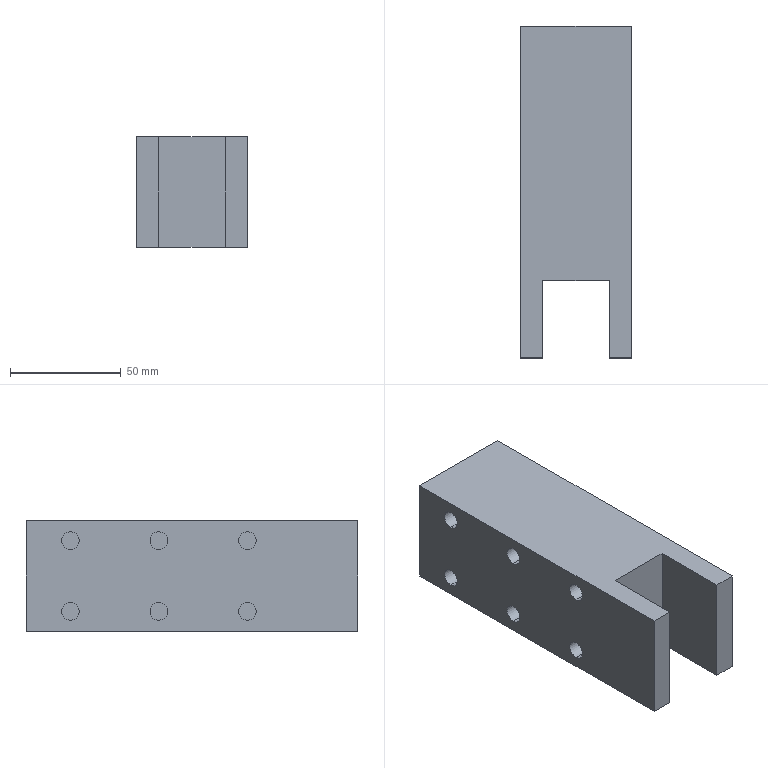Part | SolidWorks | features ICE 3, Extrusion 1, MirrorPattern 1 | 1 solid | 49 faces | box 50 x 150 x 50 mm | volume 308426 mm3 | cylinder 26 | plane 23 | commonest cylinder face diameters 8 x24 32 x2
STEP:
#1=CARTESIAN_POINT('',(-15.,130.,-20.));
#2=VERTEX_POINT('',#1);
#3=CARTESIAN_POINT('',(-15.,130.,-12.));
#4=VERTEX_POINT('',#3);
#5=CARTESIAN_POINT('',(-15.,130.,-16.));
#6=DIRECTION('',(-1.,0.,0.));
#7=DIRECTION('',(0.,0.,-1.));
#8=AXIS2_PLACEMENT_3D('',#5,#6,#7);
#9=CIRCLE('',#8,4.);
#10=EDGE_CURVE('',#2,#4,#9,.T.);
#11=ORIENTED_EDGE('',*,*,#10,.F.);
#12=CARTESIAN_POINT('',(-25.,130.,-20.));
#13=VERTEX_POINT('',#12);
#14=CARTESIAN_POINT('',(-15.,130.,-20.));
#15=DIRECTION('',(-1.,0.,0.));
#16=VECTOR('',#15,1000.);
#17=LINE('',#14,#16);
#18=EDGE_CURVE('',#2,#13,#17,.T.);
#19=ORIENTED_EDGE('',*,*,#18,.T.);
#20=CARTESIAN_POINT('',(-25.,130.,-12.));
#21=VERTEX_POINT('',#20);
#22=CARTESIAN_POINT('',(-25.,130.,-16.));
#23=DIRECTION('',(-1.,0.,0.));
#24=DIRECTION('',(0.,0.,-1.));
#25=AXIS2_PLACEMENT_3D('',#22,#23,#24);
#26=CIRCLE('',#25,4.);
#27=EDGE_CURVE('',#13,#21,#26,.T.);
#28=ORIENTED_EDGE('',*,*,#27,.T.);
#29=CARTESIAN_POINT('',(-15.,130.,-12.));
#30=DIRECTION('',(-1.,0.,0.));
#31=VECTOR('',#30,1000.);
#32=LINE('',#29,#31);
#33=EDGE_CURVE('',#4,#21,#32,.T.);
#34=ORIENTED_EDGE('',*,*,#33,.F.);
#35=EDGE_LOOP('',(#11,#19,#28,#34));
#36=FACE_OUTER_BOUND('',#35,.T.);
#37=CARTESIAN_POINT('',(-15.,130.,-16.));
#38=DIRECTION('',(-1.,0.,0.));
#39=DIRECTION('',(0.,0.,1.));
#40=AXIS2_PLACEMENT_3D('',#37,#38,#39);
#41=CYLINDRICAL_SURFACE('',#40,4.);
#42=ADVANCED_FACE('',(#36),#41,.F.);
#43=CARTESIAN_POINT('',(-15.,90.,20.));
#44=VERTEX_POINT('',#43);
#45=CARTESIAN_POINT('',(-15.,90.,12.));
#46=VERTEX_POINT('',#45);
#47=CARTESIAN_POINT('',(-15.,90.,16.));
#48=DIRECTION('',(1.,0.,0.));
#49=DIRECTION('',(0.,0.,-1.));
#50=AXIS2_PLACEMENT_3D('',#47,#48,#49);
#51=CIRCLE('',#50,4.);
#52=EDGE_CURVE('',#44,#46,#51,.T.);
#53=ORIENTED_EDGE('',*,*,#52,.T.);
#54=CARTESIAN_POINT('',(-25.,90.,12.));
#55=VERTEX_POINT('',#54);
#56=CARTESIAN_POINT('',(-15.,90.,12.));
#57=DIRECTION('',(-1.,0.,0.));
#58=VECTOR('',#57,1000.);
#59=LINE('',#56,#58);
#60=EDGE_CURVE('',#46,#55,#59,.T.);
#61=ORIENTED_EDGE('',*,*,#60,.T.);
#62=CARTESIAN_POINT('',(-25.,90.,20.));
#63=VERTEX_POINT('',#62);
#64=CARTESIAN_POINT('',(-25.,90.,16.));
#65=DIRECTION('',(1.,0.,0.));
#66=DIRECTION('',(0.,0.,-1.));
#67=AXIS2_PLACEMENT_3D('',#64,#65,#66);
#68=CIRCLE('',#67,4.);
#69=EDGE_CURVE('',#63,#55,#68,.T.);
#70=ORIENTED_EDGE('',*,*,#69,.F.);
#71=CARTESIAN_POINT('',(-15.,90.,20.));
#72=DIRECTION('',(-1.,0.,0.));
#73=VECTOR('',#72,1000.);
#74=LINE('',#71,#73);
#75=EDGE_CURVE('',#44,#63,#74,.T.);
#76=ORIENTED_EDGE('',*,*,#75,.F.);
#77=EDGE_LOOP('',(#53,#61,#70,#76));
#78=FACE_OUTER_BOUND('',#77,.T.);
#79=CARTESIAN_POINT('',(-15.,90.,16.));
#80=DIRECTION('',(-1.,0.,0.));
#81=DIRECTION('',(0.,0.,1.));
#82=AXIS2_PLACEMENT_3D('',#79,#80,#81);
#83=CYLINDRICAL_SURFACE('',#82,4.);
#84=ADVANCED_FACE('',(#78),#83,.F.);
#85=CARTESIAN_POINT('',(-15.,50.,20.));
#86=VERTEX_POINT('',#85);
#87=CARTESIAN_POINT('',(-15.,50.,12.));
#88=VERTEX_POINT('',#87);
#89=CARTESIAN_POINT('',(-15.,50.,16.));
#90=DIRECTION('',(1.,0.,0.));
#91=DIRECTION('',(0.,0.,-1.));
#92=AXIS2_PLACEMENT_3D('',#89,#90,#91);
#93=CIRCLE('',#92,4.);
#94=EDGE_CURVE('',#86,#88,#93,.T.);
#95=ORIENTED_EDGE('',*,*,#94,.T.);
#96=CARTESIAN_POINT('',(-25.,50.,12.));
#97=VERTEX_POINT('',#96);
#98=CARTESIAN_POINT('',(-15.,50.,12.));
#99=DIRECTION('',(-1.,0.,0.));
#100=VECTOR('',#99,1000.);
#101=LINE('',#98,#100);
#102=EDGE_CURVE('',#88,#97,#101,.T.);
#103=ORIENTED_EDGE('',*,*,#102,.T.);
#104=CARTESIAN_POINT('',(-25.,50.,20.));
#105=VERTEX_POINT('',#104);
#106=CARTESIAN_POINT('',(-25.,50.,16.));
#107=DIRECTION('',(1.,0.,0.));
#108=DIRECTION('',(0.,0.,-1.));
#109=AXIS2_PLACEMENT_3D('',#106,#107,#108);
#110=CIRCLE('',#109,4.);
#111=EDGE_CURVE('',#105,#97,#110,.T.);
#112=ORIENTED_EDGE('',*,*,#111,.F.);
#113=CARTESIAN_POINT('',(-15.,50.,20.));
#114=DIRECTION('',(-1.,0.,0.));
#115=VECTOR('',#114,1000.);
#116=LINE('',#113,#115);
#117=EDGE_CURVE('',#86,#105,#116,.T.);
#118=ORIENTED_EDGE('',*,*,#117,.F.);
#119=EDGE_LOOP('',(#95,#103,#112,#118));
#120=FACE_OUTER_BOUND('',#119,.T.);
#121=CARTESIAN_POINT('',(-15.,50.,16.));
#122=DIRECTION('',(-1.,0.,0.));
#123=DIRECTION('',(0.,0.,1.));
#124=AXIS2_PLACEMENT_3D('',#121,#122,#123);
#125=CYLINDRICAL_SURFACE('',#124,4.);
#126=ADVANCED_FACE('',(#120),#125,.F.);
#127=CARTESIAN_POINT('',(-15.,50.,-20.));
#128=VERTEX_POINT('',#127);
#129=CARTESIAN_POINT('',(-15.,50.,-12.));
#130=VERTEX_POINT('',#129);
#131=CARTESIAN_POINT('',(-15.,50.,-16.));
#132=DIRECTION('',(-1.,0.,0.));
#133=DIRECTION('',(0.,0.,-1.));
#134=AXIS2_PLACEMENT_3D('',#131,#132,#133);
#135=CIRCLE('',#134,4.);
#136=EDGE_CURVE('',#128,#130,#135,.T.);
#137=ORIENTED_EDGE('',*,*,#136,.F.);
#138=CARTESIAN_POINT('',(-25.,50.,-20.));
#139=VERTEX_POINT('',#138);
#140=CARTESIAN_POINT('',(-15.,50.,-20.));
#141=DIRECTION('',(-1.,0.,0.));
#142=VECTOR('',#141,1000.);
#143=LINE('',#140,#142);
#144=EDGE_CURVE('',#128,#139,#143,.T.);
#145=ORIENTED_EDGE('',*,*,#144,.T.);
#146=CARTESIAN_POINT('',(-25.,50.,-12.));
#147=VERTEX_POINT('',#146);
#148=CARTESIAN_POINT('',(-25.,50.,-16.));
#149=DIRECTION('',(-1.,0.,0.));
#150=DIRECTION('',(0.,0.,-1.));
#151=AXIS2_PLACEMENT_3D('',#148,#149,#150);
#152=CIRCLE('',#151,4.);
#153=EDGE_CURVE('',#139,#147,#152,.T.);
#154=ORIENTED_EDGE('',*,*,#153,.T.);
#155=CARTESIAN_POINT('',(-15.,50.,-12.));
#156=DIRECTION('',(-1.,0.,0.));
#157=VECTOR('',#156,1000.);
#158=LINE('',#155,#157);
#159=EDGE_CURVE('',#130,#147,#158,.T.);
#160=ORIENTED_EDGE('',*,*,#159,.F.);
#161=EDGE_LOOP('',(#137,#145,#154,#160));
#162=FACE_OUTER_BOUND('',#161,.T.);
#163=CARTESIAN_POINT('',(-15.,50.,-16.));
#164=DIRECTION('',(-1.,0.,0.));
#165=DIRECTION('',(0.,0.,1.));
#166=AXIS2_PLACEMENT_3D('',#163,#164,#165);
#167=CYLINDRICAL_SURFACE('',#166,4.);
#168=ADVANCED_FACE('',(#162),#167,.F.);
#169=CARTESIAN_POINT('',(-15.,90.,-20.));
#170=VERTEX_POINT('',#169);
#171=CARTESIAN_POINT('',(-15.,90.,-12.));
#172=VERTEX_POINT('',#171);
#173=CARTESIAN_POINT('',(-15.,90.,-16.));
#174=DIRECTION('',(-1.,0.,0.));
#175=DIRECTION('',(0.,0.,1.));
#176=AXIS2_PLACEMENT_3D('',#173,#174,#175);
#177=CIRCLE('',#176,4.);
#178=EDGE_CURVE('',#170,#172,#177,.T.);
#179=ORIENTED_EDGE('',*,*,#178,.F.);
#180=CARTESIAN_POINT('',(-25.,90.,-20.));
#181=VERTEX_POINT('',#180);
#182=CARTESIAN_POINT('',(-15.,90.,-20.));
#183=DIRECTION('',(-1.,0.,0.));
#184=VECTOR('',#183,1000.);
#185=LINE('',#182,#184);
#186=EDGE_CURVE('',#170,#181,#185,.T.);
#187=ORIENTED_EDGE('',*,*,#186,.T.);
#188=CARTESIAN_POINT('',(-25.,90.,-12.));
#189=VERTEX_POINT('',#188);
#190=CARTESIAN_POINT('',(-25.,90.,-16.));
#191=DIRECTION('',(-1.,0.,0.));
#192=DIRECTION('',(0.,0.,1.));
#193=AXIS2_PLACEMENT_3D('',#190,#191,#192);
#194=CIRCLE('',#193,4.);
#195=EDGE_CURVE('',#181,#189,#194,.T.);
#196=ORIENTED_EDGE('',*,*,#195,.T.);
#197=CARTESIAN_POINT('',(-15.,90.,-12.));
#198=DIRECTION('',(-1.,0.,0.));
#199=VECTOR('',#198,1000.);
#200=LINE('',#197,#199);
#201=EDGE_CURVE('',#172,#189,#200,.T.);
#202=ORIENTED_EDGE('',*,*,#201,.F.);
#203=EDGE_LOOP('',(#179,#187,#196,#202));
#204=FACE_OUTER_BOUND('',#203,.T.);
#205=CARTESIAN_POINT('',(-15.,90.,-16.));
#206=DIRECTION('',(-1.,0.,0.));
#207=DIRECTION('',(0.,0.,1.));
#208=AXIS2_PLACEMENT_3D('',#205,#206,#207);
#209=CYLINDRICAL_SURFACE('',#208,4.);
#210=ADVANCED_FACE('',(#204),#209,.F.);
#211=CARTESIAN_POINT('',(-15.,130.,20.));
#212=VERTEX_POINT('',#211);
#213=CARTESIAN_POINT('',(-15.,130.,12.));
#214=VERTEX_POINT('',#213);
#215=CARTESIAN_POINT('',(-15.,130.,16.));
#216=DIRECTION('',(1.,0.,0.));
#217=DIRECTION('',(0.,0.,-1.));
#218=AXIS2_PLACEMENT_3D('',#215,#216,#217);
#219=CIRCLE('',#218,4.);
#220=EDGE_CURVE('',#212,#214,#219,.T.);
#221=ORIENTED_EDGE('',*,*,#220,.T.);
#222=CARTESIAN_POINT('',(-25.,130.,12.));
#223=VERTEX_POINT('',#222);
#224=CARTESIAN_POINT('',(-15.,130.,12.));
#225=DIRECTION('',(-1.,0.,0.));
#226=VECTOR('',#225,1000.);
#227=LINE('',#224,#226);
#228=EDGE_CURVE('',#214,#223,#227,.T.);
#229=ORIENTED_EDGE('',*,*,#228,.T.);
#230=CARTESIAN_POINT('',(-25.,130.,20.));
#231=VERTEX_POINT('',#230);
#232=CARTESIAN_POINT('',(-25.,130.,16.));
#233=DIRECTION('',(1.,0.,0.));
#234=DIRECTION('',(0.,0.,-1.));
#235=AXIS2_PLACEMENT_3D('',#232,#233,#234);
#236=CIRCLE('',#235,4.);
#237=EDGE_CURVE('',#231,#223,#236,.T.);
#238=ORIENTED_EDGE('',*,*,#237,.F.);
#239=CARTESIAN_POINT('',(-15.,130.,20.));
#240=DIRECTION('',(-1.,0.,0.));
#241=VECTOR('',#240,1000.);
#242=LINE('',#239,#241);
#243=EDGE_CURVE('',#212,#231,#242,.T.);
#244=ORIENTED_EDGE('',*,*,#243,.F.);
#245=EDGE_LOOP('',(#221,#229,#238,#244));
#246=FACE_OUTER_BOUND('',#245,.T.);
#247=CARTESIAN_POINT('',(-15.,130.,16.));
#248=DIRECTION('',(-1.,0.,0.));
#249=DIRECTION('',(0.,0.,1.));
#250=AXIS2_PLACEMENT_3D('',#247,#248,#249);
#251=CYLINDRICAL_SURFACE('',#250,4.);
#252=ADVANCED_FACE('',(#246),#251,.F.);
#253=CARTESIAN_POINT('',(15.,130.,-20.));
#254=VERTEX_POINT('',#253);
#255=CARTESIAN_POINT('',(15.,130.,-12.));
#256=VERTEX_POINT('',#255);
#257=CARTESIAN_POINT('',(15.,130.,-16.));
#258=DIRECTION('',(-1.,0.,0.));
#259=DIRECTION('',(0.,0.,-1.));
#260=AXIS2_PLACEMENT_3D('',#257,#258,#259);
#261=CIRCLE('',#260,4.);
#262=EDGE_CURVE('',#254,#256,#261,.T.);
#263=ORIENTED_EDGE('',*,*,#262,.T.);
#264=CARTESIAN_POINT('',(25.,130.,-12.));
#265=VERTEX_POINT('',#264);
#266=CARTESIAN_POINT('',(15.,130.,-12.));
#267=DIRECTION('',(1.,0.,0.));
#268=VECTOR('',#267,1000.);
#269=LINE('',#266,#268);
#270=EDGE_CURVE('',#256,#265,#269,.T.);
#271=ORIENTED_EDGE('',*,*,#270,.T.);
#272=CARTESIAN_POINT('',(25.,130.,-20.));
#273=VERTEX_POINT('',#272);
#274=CARTESIAN_POINT('',(25.,130.,-16.));
#275=DIRECTION('',(-1.,0.,0.));
#276=DIRECTION('',(0.,0.,-1.));
#277=AXIS2_PLACEMENT_3D('',#274,#275,#276);
#278=CIRCLE('',#277,4.);
#279=EDGE_CURVE('',#273,#265,#278,.T.);
#280=ORIENTED_EDGE('',*,*,#279,.F.);
#281=CARTESIAN_POINT('',(15.,130.,-20.));
#282=DIRECTION('',(1.,0.,0.));
#283=VECTOR('',#282,1000.);
#284=LINE('',#281,#283);
#285=EDGE_CURVE('',#254,#273,#284,.T.);
#286=ORIENTED_EDGE('',*,*,#285,.F.);
#287=EDGE_LOOP('',(#263,#271,#280,#286));
#288=FACE_OUTER_BOUND('',#287,.T.);
#289=CARTESIAN_POINT('',(15.,130.,-16.));
#290=DIRECTION('',(1.,0.,0.));
#291=DIRECTION('',(0.,0.,-1.));
#292=AXIS2_PLACEMENT_3D('',#289,#290,#291);
#293=CYLINDRICAL_SURFACE('',#292,4.);
#294=ADVANCED_FACE('',(#288),#293,.F.);
#295=CARTESIAN_POINT('',(15.,90.,20.));
#296=VERTEX_POINT('',#295);
#297=CARTESIAN_POINT('',(15.,90.,12.));
#298=VERTEX_POINT('',#297);
#299=CARTESIAN_POINT('',(15.,90.,16.));
#300=DIRECTION('',(1.,0.,0.));
#301=DIRECTION('',(0.,0.,-1.));
#302=AXIS2_PLACEMENT_3D('',#299,#300,#301);
#303=CIRCLE('',#302,4.);
#304=EDGE_CURVE('',#296,#298,#303,.T.);
#305=ORIENTED_EDGE('',*,*,#304,.F.);
#306=CARTESIAN_POINT('',(25.,90.,20.));
#307=VERTEX_POINT('',#306);
#308=CARTESIAN_POINT('',(15.,90.,20.));
#309=DIRECTION('',(1.,0.,0.));
#310=VECTOR('',#309,1000.);
#311=LINE('',#308,#310);
#312=EDGE_CURVE('',#296,#307,#311,.T.);
#313=ORIENTED_EDGE('',*,*,#312,.T.);
#314=CARTESIAN_POINT('',(25.,90.,12.));
#315=VERTEX_POINT('',#314);
#316=CARTESIAN_POINT('',(25.,90.,16.));
#317=DIRECTION('',(1.,0.,0.));
#318=DIRECTION('',(0.,0.,-1.));
#319=AXIS2_PLACEMENT_3D('',#316,#317,#318);
#320=CIRCLE('',#319,4.);
#321=EDGE_CURVE('',#307,#315,#320,.T.);
#322=ORIENTED_EDGE('',*,*,#321,.T.);
#323=CARTESIAN_POINT('',(15.,90.,12.));
#324=DIRECTION('',(1.,0.,0.));
#325=VECTOR('',#324,1000.);
#326=LINE('',#323,#325);
#327=EDGE_CURVE('',#298,#315,#326,.T.);
#328=ORIENTED_EDGE('',*,*,#327,.F.);
#329=EDGE_LOOP('',(#305,#313,#322,#328));
#330=FACE_OUTER_BOUND('',#329,.T.);
#331=CARTESIAN_POINT('',(15.,90.,16.));
#332=DIRECTION('',(1.,0.,0.));
#333=DIRECTION('',(0.,0.,-1.));
#334=AXIS2_PLACEMENT_3D('',#331,#332,#333);
#335=CYLINDRICAL_SURFACE('',#334,4.);
#336=ADVANCED_FACE('',(#330),#335,.F.);
#337=CARTESIAN_POINT('',(15.,50.,20.));
#338=VERTEX_POINT('',#337);
#339=CARTESIAN_POINT('',(15.,50.,12.));
#340=VERTEX_POINT('',#339);
#341=CARTESIAN_POINT('',(15.,50.,16.));
#342=DIRECTION('',(1.,0.,0.));
#343=DIRECTION('',(0.,0.,-1.));
#344=AXIS2_PLACEMENT_3D('',#341,#342,#343);
#345=CIRCLE('',#344,4.);
#346=EDGE_CURVE('',#338,#340,#345,.T.);
#347=ORIENTED_EDGE('',*,*,#346,.F.);
#348=CARTESIAN_POINT('',(25.,50.,20.));
#349=VERTEX_POINT('',#348);
#350=CARTESIAN_POINT('',(15.,50.,20.));
#351=DIRECTION('',(1.,0.,0.));
#352=VECTOR('',#351,1000.);
#353=LINE('',#350,#352);
#354=EDGE_CURVE('',#338,#349,#353,.T.);
#355=ORIENTED_EDGE('',*,*,#354,.T.);
#356=CARTESIAN_POINT('',(25.,50.,12.));
#357=VERTEX_POINT('',#356);
#358=CARTESIAN_POINT('',(25.,50.,16.));
#359=DIRECTION('',(1.,0.,0.));
#360=DIRECTION('',(0.,0.,-1.));
#361=AXIS2_PLACEMENT_3D('',#358,#359,#360);
#362=CIRCLE('',#361,4.);
#363=EDGE_CURVE('',#349,#357,#362,.T.);
#364=ORIENTED_EDGE('',*,*,#363,.T.);
#365=CARTESIAN_POINT('',(15.,50.,12.));
#366=DIRECTION('',(1.,0.,0.));
#367=VECTOR('',#366,1000.);
#368=LINE('',#365,#367);
#369=EDGE_CURVE('',#340,#357,#368,.T.);
#370=ORIENTED_EDGE('',*,*,#369,.F.);
#371=EDGE_LOOP('',(#347,#355,#364,#370));
#372=FACE_OUTER_BOUND('',#371,.T.);
#373=CARTESIAN_POINT('',(15.,50.,16.));
#374=DIRECTION('',(1.,0.,0.));
#375=DIRECTION('',(0.,0.,-1.));
#376=AXIS2_PLACEMENT_3D('',#373,#374,#375);
#377=CYLINDRICAL_SURFACE('',#376,4.);
#378=ADVANCED_FACE('',(#372),#377,.F.);
#379=CARTESIAN_POINT('',(15.,50.,-20.));
#380=VERTEX_POINT('',#379);
#381=CARTESIAN_POINT('',(15.,50.,-12.));
#382=VERTEX_POINT('',#381);
#383=CARTESIAN_POINT('',(15.,50.,-16.));
#384=DIRECTION('',(-1.,0.,0.));
#385=DIRECTION('',(0.,0.,-1.));
#386=AXIS2_PLACEMENT_3D('',#383,#384,#385);
#387=CIRCLE('',#386,4.);
#388=EDGE_CURVE('',#380,#382,#387,.T.);
#389=ORIENTED_EDGE('',*,*,#388,.T.);
#390=CARTESIAN_POINT('',(25.,50.,-12.));
#391=VERTEX_POINT('',#390);
#392=CARTESIAN_POINT('',(15.,50.,-12.));
#393=DIRECTION('',(1.,0.,0.));
#394=VECTOR('',#393,1000.);
#395=LINE('',#392,#394);
#396=EDGE_CURVE('',#382,#391,#395,.T.);
#397=ORIENTED_EDGE('',*,*,#396,.T.);
#398=CARTESIAN_POINT('',(25.,50.,-20.));
#399=VERTEX_POINT('',#398);
#400=CARTESIAN_POINT('',(25.,50.,-16.));
#401=DIRECTION('',(-1.,0.,0.));
#402=DIRECTION('',(0.,0.,-1.));
#403=AXIS2_PLACEMENT_3D('',#400,#401,#402);
#404=CIRCLE('',#403,4.);
#405=EDGE_CURVE('',#399,#391,#404,.T.);
#406=ORIENTED_EDGE('',*,*,#405,.F.);
#407=CARTESIAN_POINT('',(15.,50.,-20.));
#408=DIRECTION('',(1.,0.,0.));
#409=VECTOR('',#408,1000.);
#410=LINE('',#407,#409);
#411=EDGE_CURVE('',#380,#399,#410,.T.);
#412=ORIENTED_EDGE('',*,*,#411,.F.);
#413=EDGE_LOOP('',(#389,#397,#406,#412));
#414=FACE_OUTER_BOUND('',#413,.T.);
#415=CARTESIAN_POINT('',(15.,50.,-16.));
#416=DIRECTION('',(1.,0.,0.));
#417=DIRECTION('',(0.,0.,-1.));
#418=AXIS2_PLACEMENT_3D('',#415,#416,#417);
#419=CYLINDRICAL_SURFACE('',#418,4.);
#420=ADVANCED_FACE('',(#414),#419,.F.);
#421=CARTESIAN_POINT('',(15.,90.,-20.));
#422=VERTEX_POINT('',#421);
#423=CARTESIAN_POINT('',(15.,90.,-12.));
#424=VERTEX_POINT('',#423);
#425=CARTESIAN_POINT('',(15.,90.,-16.));
#426=DIRECTION('',(-1.,0.,0.));
#427=DIRECTION('',(0.,0.,1.));
#428=AXIS2_PLACEMENT_3D('',#425,#426,#427);
#429=CIRCLE('',#428,4.);
#430=EDGE_CURVE('',#422,#424,#429,.T.);
#431=ORIENTED_EDGE('',*,*,#430,.T.);
#432=CARTESIAN_POINT('',(25.,90.,-12.));
#433=VERTEX_POINT('',#432);
#434=CARTESIAN_POINT('',(15.,90.,-12.));
#435=DIRECTION('',(1.,0.,0.));
#436=VECTOR('',#435,1000.);
#437=LINE('',#434,#436);
#438=EDGE_CURVE('',#424,#433,#437,.T.);
#439=ORIENTED_EDGE('',*,*,#438,.T.);
#440=CARTESIAN_POINT('',(25.,90.,-20.));
#441=VERTEX_POINT('',#440);
#442=CARTESIAN_POINT('',(25.,90.,-16.));
#443=DIRECTION('',(-1.,0.,0.));
#444=DIRECTION('',(0.,0.,1.));
#445=AXIS2_PLACEMENT_3D('',#442,#443,#444);
#446=CIRCLE('',#445,4.);
#447=EDGE_CURVE('',#441,#433,#446,.T.);
#448=ORIENTED_EDGE('',*,*,#447,.F.);
#449=CARTESIAN_POINT('',(15.,90.,-20.));
#450=DIRECTION('',(1.,0.,0.));
#451=VECTOR('',#450,1000.);
#452=LINE('',#449,#451);
#453=EDGE_CURVE('',#422,#441,#452,.T.);
#454=ORIENTED_EDGE('',*,*,#453,.F.);
#455=EDGE_LOOP('',(#431,#439,#448,#454));
#456=FACE_OUTER_BOUND('',#455,.T.);
#457=CARTESIAN_POINT('',(15.,90.,-16.));
#458=DIRECTION('',(1.,0.,0.));
#459=DIRECTION('',(0.,0.,-1.));
#460=AXIS2_PLACEMENT_3D('',#457,#458,#459);
#461=CYLINDRICAL_SURFACE('',#460,4.);
#462=ADVANCED_FACE('',(#456),#461,.F.);
#463=CARTESIAN_POINT('',(15.,130.,20.));
#464=VERTEX_POINT('',#463);
#465=CARTESIAN_POINT('',(15.,130.,12.));
#466=VERTEX_POINT('',#465);
#467=CARTESIAN_POINT('',(15.,130.,16.));
#468=DIRECTION('',(1.,0.,0.));
#469=DIRECTION('',(0.,0.,-1.));
#470=AXIS2_PLACEMENT_3D('',#467,#468,#469);
#471=CIRCLE('',#470,4.);
#472=EDGE_CURVE('',#464,#466,#471,.T.);
#473=ORIENTED_EDGE('',*,*,#472,.F.);
#474=CARTESIAN_POINT('',(25.,130.,20.));
#475=VERTEX_POINT('',#474);
#476=CARTESIAN_POINT('',(15.,130.,20.));
#477=DIRECTION('',(1.,0.,0.));
#478=VECTOR('',#477,1000.);
#479=LINE('',#476,#478);
#480=EDGE_CURVE('',#464,#475,#479,.T.);
#481=ORIENTED_EDGE('',*,*,#480,.T.);
#482=CARTESIAN_POINT('',(25.,130.,12.));
#483=VERTEX_POINT('',#482);
#484=CARTESIAN_POINT('',(25.,130.,16.));
#485=DIRECTION('',(1.,0.,0.));
#486=DIRECTION('',(0.,0.,-1.));
#487=AXIS2_PLACEMENT_3D('',#484,#485,#486);
#488=CIRCLE('',#487,4.);
#489=EDGE_CURVE('',#475,#483,#488,.T.);
#490=ORIENTED_EDGE('',*,*,#489,.T.);
#491=CARTESIAN_POINT('',(15.,130.,12.));
#492=DIRECTION('',(1.,0.,0.));
#493=VECTOR('',#492,1000.);
#494=LINE('',#491,#493);
#495=EDGE_CURVE('',#466,#483,#494,.T.);
#496=ORIENTED_EDGE('',*,*,#495,.F.);
#497=EDGE_LOOP('',(#473,#481,#490,#496));
#498=FACE_OUTER_BOUND('',#497,.T.);
#499=CARTESIAN_POINT('',(15.,130.,16.));
#500=DIRECTION('',(1.,0.,0.));
#501=DIRECTION('',(0.,0.,-1.));
#502=AXIS2_PLACEMENT_3D('',#499,#500,#501);
#503=CYLINDRICAL_SURFACE('',#502,4.);
#504=ADVANCED_FACE('',(#498),#503,.F.);
#505=CARTESIAN_POINT('',(0.,140.,-16.));
#506=VERTEX_POINT('',#505);
#507=CARTESIAN_POINT('',(0.,140.,16.));
#508=VERTEX_POINT('',#507);
#509=CARTESIAN_POINT('',(0.,140.,0.));
#510=DIRECTION('',(0.,1.,0.));
#511=DIRECTION('',(0.,0.,1.));
#512=AXIS2_PLACEMENT_3D('',#509,#510,#511);
#513=CIRCLE('',#512,16.);
#514=EDGE_CURVE('',#506,#508,#513,.T.);
#515=ORIENTED_EDGE('',*,*,#514,.F.);
#516=CARTESIAN_POINT('',(0.,150.,-16.));
#517=VERTEX_POINT('',#516);
#518=CARTESIAN_POINT('',(0.,140.,-16.));
#519=DIRECTION('',(0.,1.,0.));
#520=VECTOR('',#519,1000.);
#521=LINE('',#518,#520);
#522=EDGE_CURVE('',#506,#517,#521,.T.);
#523=ORIENTED_EDGE('',*,*,#522,.T.);
#524=CARTESIAN_POINT('',(0.,150.,16.));
#525=VERTEX_POINT('',#524);
#526=CARTESIAN_POINT('',(0.,150.,0.));
#527=DIRECTION('',(0.,1.,0.));
#528=DIRECTION('',(0.,0.,1.));
#529=AXIS2_PLACEMENT_3D('',#526,#527,#528);
#530=CIRCLE('',#529,16.);
#531=EDGE_CURVE('',#517,#525,#530,.T.);
#532=ORIENTED_EDGE('',*,*,#531,.T.);
#533=CARTESIAN_POINT('',(0.,140.,16.));
#534=DIRECTION('',(0.,1.,0.));
#535=VECTOR('',#534,1000.);
#536=LINE('',#533,#535);
#537=EDGE_CURVE('',#508,#525,#536,.T.);
#538=ORIENTED_EDGE('',*,*,#537,.F.);
#539=EDGE_LOOP('',(#515,#523,#532,#538));
#540=FACE_OUTER_BOUND('',#539,.T.);
#541=CARTESIAN_POINT('',(0.,140.,0.));
#542=DIRECTION('',(0.,1.,0.));
#543=DIRECTION('',(0.,0.,1.));
#544=AXIS2_PLACEMENT_3D('',#541,#542,#543);
#545=CYLINDRICAL_SURFACE('',#544,16.);
#546=ADVANCED_FACE('',(#540),#545,.F.);
#547=CARTESIAN_POINT('',(-25.,50.,-16.));
#548=DIRECTION('',(-1.,0.,0.));
#549=DIRECTION('',(0.,0.,-1.));
#550=AXIS2_PLACEMENT_3D('',#547,#548,#549);
#551=CIRCLE('',#550,4.);
#552=EDGE_CURVE('',#147,#139,#551,.T.);
#553=ORIENTED_EDGE('',*,*,#552,.F.);
#554=ORIENTED_EDGE('',*,*,#153,.F.);
#555=EDGE_LOOP('',(#553,#554));
#556=FACE_BOUND('',#555,.T.);
#557=CARTESIAN_POINT('',(-25.,0.,-25.));
#558=VERTEX_POINT('',#557);
#559=CARTESIAN_POINT('',(-25.,0.,25.));
#560=VERTEX_POINT('',#559);
#561=CARTESIAN_POINT('',(-25.,0.,-25.));
#562=DIRECTION('',(0.,0.,1.));
#563=VECTOR('',#562,1000.);
#564=LINE('',#561,#563);
#565=EDGE_CURVE('',#558,#560,#564,.T.);
#566=ORIENTED_EDGE('',*,*,#565,.T.);
#567=CARTESIAN_POINT('',(-25.,150.,25.));
#568=VERTEX_POINT('',#567);
#569=CARTESIAN_POINT('',(-25.,150.,25.));
#570=DIRECTION('',(0.,-1.,0.));
#571=VECTOR('',#570,1000.);
#572=LINE('',#569,#571);
#573=EDGE_CURVE('',#568,#560,#572,.T.);
#574=ORIENTED_EDGE('',*,*,#573,.F.);
#575=CARTESIAN_POINT('',(-25.,150.,-25.));
#576=VERTEX_POINT('',#575);
#577=CARTESIAN_POINT('',(-25.,150.,-25.));
#578=DIRECTION('',(0.,0.,1.));
#579=VECTOR('',#578,1000.);
#580=LINE('',#577,#579);
#581=EDGE_CURVE('',#576,#568,#580,.T.);
#582=ORIENTED_EDGE('',*,*,#581,.F.);
#583=CARTESIAN_POINT('',(-25.,150.,-25.));
#584=DIRECTION('',(0.,-1.,0.));
#585=VECTOR('',#584,1000.);
#586=LINE('',#583,#585);
#587=EDGE_CURVE('',#576,#558,#586,.T.);
#588=ORIENTED_EDGE('',*,*,#587,.T.);
#589=EDGE_LOOP('',(#566,#574,#582,#588));
#590=FACE_OUTER_BOUND('',#589,.T.);
#591=ORIENTED_EDGE('',*,*,#237,.T.);
#592=CARTESIAN_POINT('',(-25.,130.,16.));
#593=DIRECTION('',(1.,0.,0.));
#594=DIRECTION('',(0.,0.,-1.));
#595=AXIS2_PLACEMENT_3D('',#592,#593,#594);
#596=CIRCLE('',#595,4.);
#597=EDGE_CURVE('',#223,#231,#596,.T.);
#598=ORIENTED_EDGE('',*,*,#597,.T.);
#599=EDGE_LOOP('',(#591,#598));
#600=FACE_BOUND('',#599,.T.);
#601=CARTESIAN_POINT('',(-25.,90.,-16.));
#602=DIRECTION('',(-1.,0.,0.));
#603=DIRECTION('',(0.,0.,1.));
#604=AXIS2_PLACEMENT_3D('',#601,#602,#603);
#605=CIRCLE('',#604,4.);
#606=EDGE_CURVE('',#189,#181,#605,.T.);
#607=ORIENTED_EDGE('',*,*,#606,.F.);
#608=ORIENTED_EDGE('',*,*,#195,.F.);
#609=EDGE_LOOP('',(#607,#608));
#610=FACE_BOUND('',#609,.T.);
#611=ORIENTED_EDGE('',*,*,#111,.T.);
#612=CARTESIAN_POINT('',(-25.,50.,16.));
#613=DIRECTION('',(1.,0.,0.));
#614=DIRECTION('',(0.,0.,-1.));
#615=AXIS2_PLACEMENT_3D('',#612,#613,#614);
#616=CIRCLE('',#615,4.);
#617=EDGE_CURVE('',#97,#105,#616,.T.);
#618=ORIENTED_EDGE('',*,*,#617,.T.);
#619=EDGE_LOOP('',(#611,#618));
#620=FACE_BOUND('',#619,.T.);
#621=ORIENTED_EDGE('',*,*,#69,.T.);
#622=CARTESIAN_POINT('',(-25.,90.,16.));
#623=DIRECTION('',(1.,0.,0.));
#624=DIRECTION('',(0.,0.,-1.));
#625=AXIS2_PLACEMENT_3D('',#622,#623,#624);
#626=CIRCLE('',#625,4.);
#627=EDGE_CURVE('',#55,#63,#626,.T.);
#628=ORIENTED_EDGE('',*,*,#627,.T.);
#629=EDGE_LOOP('',(#621,#628));
#630=FACE_BOUND('',#629,.T.);
#631=CARTESIAN_POINT('',(-25.,130.,-16.));
#632=DIRECTION('',(-1.,0.,0.));
#633=DIRECTION('',(0.,0.,-1.));
#634=AXIS2_PLACEMENT_3D('',#631,#632,#633);
#635=CIRCLE('',#634,4.);
#636=EDGE_CURVE('',#21,#13,#635,.T.);
#637=ORIENTED_EDGE('',*,*,#636,.F.);
#638=ORIENTED_EDGE('',*,*,#27,.F.);
#639=EDGE_LOOP('',(#637,#638));
#640=FACE_BOUND('',#639,.T.);
#641=CARTESIAN_POINT('',(-25.,150.,-25.));
#642=DIRECTION('',(1.,0.,0.));
#643=DIRECTION('',(0.,0.,-1.));
#644=AXIS2_PLACEMENT_3D('',#641,#642,#643);
#645=PLANE('',#644);
#646=ADVANCED_FACE('',(#556,#590,#600,#610,#620,#630,#640),#645,.F.);
#647=CARTESIAN_POINT('',(25.,90.,16.));
#648=DIRECTION('',(1.,0.,0.));
#649=DIRECTION('',(0.,0.,-1.));
#650=AXIS2_PLACEMENT_3D('',#647,#648,#649);
#651=CIRCLE('',#650,4.);
#652=EDGE_CURVE('',#315,#307,#651,.T.);
#653=ORIENTED_EDGE('',*,*,#652,.F.);
#654=ORIENTED_EDGE('',*,*,#321,.F.);
#655=EDGE_LOOP('',(#653,#654));
#656=FACE_BOUND('',#655,.T.);
#657=CARTESIAN_POINT('',(25.,50.,16.));
#658=DIRECTION('',(1.,0.,0.));
#659=DIRECTION('',(0.,0.,-1.));
#660=AXIS2_PLACEMENT_3D('',#657,#658,#659);
#661=CIRCLE('',#660,4.);
#662=EDGE_CURVE('',#357,#349,#661,.T.);
#663=ORIENTED_EDGE('',*,*,#662,.F.);
#664=ORIENTED_EDGE('',*,*,#363,.F.);
#665=EDGE_LOOP('',(#663,#664));
#666=FACE_BOUND('',#665,.T.);
#667=CARTESIAN_POINT('',(25.,130.,16.));
#668=DIRECTION('',(1.,0.,0.));
#669=DIRECTION('',(0.,0.,-1.));
#670=AXIS2_PLACEMENT_3D('',#667,#668,#669);
#671=CIRCLE('',#670,4.);
#672=EDGE_CURVE('',#483,#475,#671,.T.);
#673=ORIENTED_EDGE('',*,*,#672,.F.);
#674=ORIENTED_EDGE('',*,*,#489,.F.);
#675=EDGE_LOOP('',(#673,#674));
#676=FACE_BOUND('',#675,.T.);
#677=CARTESIAN_POINT('',(25.,0.,25.));
#678=VERTEX_POINT('',#677);
#679=CARTESIAN_POINT('',(25.,0.,-25.));
#680=VERTEX_POINT('',#679);
#681=CARTESIAN_POINT('',(25.,0.,-25.));
#682=DIRECTION('',(0.,0.,-1.));
#683=VECTOR('',#682,1000.);
#684=LINE('',#681,#683);
#685=EDGE_CURVE('',#678,#680,#684,.T.);
#686=ORIENTED_EDGE('',*,*,#685,.T.);
#687=CARTESIAN_POINT('',(25.,150.,-25.));
#688=VERTEX_POINT('',#687);
#689=CARTESIAN_POINT('',(25.,150.,-25.));
#690=DIRECTION('',(0.,-1.,0.));
#691=VECTOR('',#690,1000.);
#692=LINE('',#689,#691);
#693=EDGE_CURVE('',#688,#680,#692,.T.);
#694=ORIENTED_EDGE('',*,*,#693,.F.);
#695=CARTESIAN_POINT('',(25.,150.,25.));
#696=VERTEX_POINT('',#695);
#697=CARTESIAN_POINT('',(25.,150.,-25.));
#698=DIRECTION('',(0.,0.,-1.));
#699=VECTOR('',#698,1000.);
#700=LINE('',#697,#699);
#701=EDGE_CURVE('',#696,#688,#700,.T.);
#702=ORIENTED_EDGE('',*,*,#701,.F.);
#703=CARTESIAN_POINT('',(25.,150.,25.));
#704=DIRECTION('',(0.,-1.,0.));
#705=VECTOR('',#704,1000.);
#706=LINE('',#703,#705);
#707=EDGE_CURVE('',#696,#678,#706,.T.);
#708=ORIENTED_EDGE('',*,*,#707,.T.);
#709=EDGE_LOOP('',(#686,#694,#702,#708));
#710=FACE_OUTER_BOUND('',#709,.T.);
#711=ORIENTED_EDGE('',*,*,#447,.T.);
#712=CARTESIAN_POINT('',(25.,90.,-16.));
#713=DIRECTION('',(-1.,0.,0.));
#714=DIRECTION('',(0.,0.,1.));
#715=AXIS2_PLACEMENT_3D('',#712,#713,#714);
#716=CIRCLE('',#715,4.);
#717=EDGE_CURVE('',#433,#441,#716,.T.);
#718=ORIENTED_EDGE('',*,*,#717,.T.);
#719=EDGE_LOOP('',(#711,#718));
#720=FACE_BOUND('',#719,.T.);
#721=ORIENTED_EDGE('',*,*,#405,.T.);
#722=CARTESIAN_POINT('',(25.,50.,-16.));
#723=DIRECTION('',(-1.,0.,0.));
#724=DIRECTION('',(0.,0.,-1.));
#725=AXIS2_PLACEMENT_3D('',#722,#723,#724);
#726=CIRCLE('',#725,4.);
#727=EDGE_CURVE('',#391,#399,#726,.T.);
#728=ORIENTED_EDGE('',*,*,#727,.T.);
#729=EDGE_LOOP('',(#721,#728));
#730=FACE_BOUND('',#729,.T.);
#731=ORIENTED_EDGE('',*,*,#279,.T.);
#732=CARTESIAN_POINT('',(25.,130.,-16.));
#733=DIRECTION('',(-1.,0.,0.));
#734=DIRECTION('',(0.,0.,-1.));
#735=AXIS2_PLACEMENT_3D('',#732,#733,#734);
#736=CIRCLE('',#735,4.);
#737=EDGE_CURVE('',#265,#273,#736,.T.);
#738=ORIENTED_EDGE('',*,*,#737,.T.);
#739=EDGE_LOOP('',(#731,#738));
#740=FACE_BOUND('',#739,.T.);
#741=CARTESIAN_POINT('',(25.,150.,-25.));
#742=DIRECTION('',(-1.,0.,0.));
#743=DIRECTION('',(0.,0.,1.));
#744=AXIS2_PLACEMENT_3D('',#741,#742,#743);
#745=PLANE('',#744);
#746=ADVANCED_FACE('',(#656,#666,#676,#710,#720,#730,#740),#745,.F.);
#747=CARTESIAN_POINT('',(15.,0.,25.));
#748=VERTEX_POINT('',#747);
#749=CARTESIAN_POINT('',(-25.,0.,25.));
#750=DIRECTION('',(1.,0.,0.));
#751=VECTOR('',#750,1000.);
#752=LINE('',#749,#751);
#753=EDGE_CURVE('',#748,#678,#752,.T.);
#754=ORIENTED_EDGE('',*,*,#753,.F.);
#755=CARTESIAN_POINT('',(15.,0.,-25.));
#756=VERTEX_POINT('',#755);
#757=CARTESIAN_POINT('',(15.,0.,25.));
#758=DIRECTION('',(0.,0.,1.));
#759=VECTOR('',#758,1000.);
#760=LINE('',#757,#759);
#761=EDGE_CURVE('',#756,#748,#760,.T.);
#762=ORIENTED_EDGE('',*,*,#761,.F.);
#763=CARTESIAN_POINT('',(-25.,0.,-25.));
#764=DIRECTION('',(-1.,0.,0.));
#765=VECTOR('',#764,1000.);
#766=LINE('',#763,#765);
#767=EDGE_CURVE('',#680,#756,#766,.T.);
#768=ORIENTED_EDGE('',*,*,#767,.F.);
#769=ORIENTED_EDGE('',*,*,#685,.F.);
#770=EDGE_LOOP('',(#754,#762,#768,#769));
#771=FACE_OUTER_BOUND('',#770,.T.);
#772=CARTESIAN_POINT('',(0.,0.,0.));
#773=DIRECTION('',(0.,1.,0.));
#774=DIRECTION('',(0.,0.,1.));
#775=AXIS2_PLACEMENT_3D('',#772,#773,#774);
#776=PLANE('',#775);
#777=ADVANCED_FACE('',(#771),#776,.F.);
#778=ORIENTED_EDGE('',*,*,#767,.T.);
#779=CARTESIAN_POINT('',(15.,35.,-25.));
#780=VERTEX_POINT('',#779);
#781=CARTESIAN_POINT('',(15.,35.,-25.));
#782=DIRECTION('',(0.,-1.,0.));
#783=VECTOR('',#782,1000.);
#784=LINE('',#781,#783);
#785=EDGE_CURVE('',#780,#756,#784,.T.);
#786=ORIENTED_EDGE('',*,*,#785,.F.);
#787=CARTESIAN_POINT('',(-15.,35.,-25.));
#788=VERTEX_POINT('',#787);
#789=CARTESIAN_POINT('',(-15.,35.,-25.));
#790=DIRECTION('',(1.,0.,0.));
#791=VECTOR('',#790,1000.);
#792=LINE('',#789,#791);
#793=EDGE_CURVE('',#788,#780,#792,.T.);
#794=ORIENTED_EDGE('',*,*,#793,.F.);
#795=CARTESIAN_POINT('',(-15.,0.,-25.));
#796=VERTEX_POINT('',#795);
#797=CARTESIAN_POINT('',(-15.,35.,-25.));
#798=DIRECTION('',(0.,-1.,0.));
#799=VECTOR('',#798,1000.);
#800=LINE('',#797,#799);
#801=EDGE_CURVE('',#788,#796,#800,.T.);
#802=ORIENTED_EDGE('',*,*,#801,.T.);
#803=CARTESIAN_POINT('',(-25.,0.,-25.));
#804=DIRECTION('',(-1.,0.,0.));
#805=VECTOR('',#804,1000.);
#806=LINE('',#803,#805);
#807=EDGE_CURVE('',#796,#558,#806,.T.);
#808=ORIENTED_EDGE('',*,*,#807,.T.);
#809=ORIENTED_EDGE('',*,*,#587,.F.);
#810=CARTESIAN_POINT('',(-25.,150.,-25.));
#811=DIRECTION('',(-1.,0.,0.));
#812=VECTOR('',#811,1000.);
#813=LINE('',#810,#812);
#814=EDGE_CURVE('',#688,#576,#813,.T.);
#815=ORIENTED_EDGE('',*,*,#814,.F.);
#816=ORIENTED_EDGE('',*,*,#693,.T.);
#817=EDGE_LOOP('',(#778,#786,#794,#802,#808,#809,#815,#816));
#818=FACE_OUTER_BOUND('',#817,.T.);
#819=CARTESIAN_POINT('',(-25.,150.,-25.));
#820=DIRECTION('',(0.,0.,1.));
#821=DIRECTION('',(1.,0.,0.));
#822=AXIS2_PLACEMENT_3D('',#819,#820,#821);
#823=PLANE('',#822);
#824=ADVANCED_FACE('',(#818),#823,.F.);
#825=CARTESIAN_POINT('',(15.,35.,25.));
#826=VERTEX_POINT('',#825);
#827=CARTESIAN_POINT('',(-15.,35.,25.));
#828=VERTEX_POINT('',#827);
#829=CARTESIAN_POINT('',(-15.,35.,25.));
#830=DIRECTION('',(-1.,0.,0.));
#831=VECTOR('',#830,1000.);
#832=LINE('',#829,#831);
#833=EDGE_CURVE('',#826,#828,#832,.T.);
#834=ORIENTED_EDGE('',*,*,#833,.F.);
#835=CARTESIAN_POINT('',(15.,35.,25.));
#836=DIRECTION('',(0.,-1.,0.));
#837=VECTOR('',#836,1000.);
#838=LINE('',#835,#837);
#839=EDGE_CURVE('',#826,#748,#838,.T.);
#840=ORIENTED_EDGE('',*,*,#839,.T.);
#841=ORIENTED_EDGE('',*,*,#753,.T.);
#842=ORIENTED_EDGE('',*,*,#707,.F.);
#843=CARTESIAN_POINT('',(-25.,150.,25.));
#844=DIRECTION('',(1.,0.,0.));
#845=VECTOR('',#844,1000.);
#846=LINE('',#843,#845);
#847=EDGE_CURVE('',#568,#696,#846,.T.);
#848=ORIENTED_EDGE('',*,*,#847,.F.);
#849=ORIENTED_EDGE('',*,*,#573,.T.);
#850=CARTESIAN_POINT('',(-15.,0.,25.));
#851=VERTEX_POINT('',#850);
#852=CARTESIAN_POINT('',(-25.,0.,25.));
#853=DIRECTION('',(1.,0.,0.));
#854=VECTOR('',#853,1000.);
#855=LINE('',#852,#854);
#856=EDGE_CURVE('',#560,#851,#855,.T.);
#857=ORIENTED_EDGE('',*,*,#856,.T.);
#858=CARTESIAN_POINT('',(-15.,35.,25.));
#859=DIRECTION('',(0.,-1.,0.));
#860=VECTOR('',#859,1000.);
#861=LINE('',#858,#860);
#862=EDGE_CURVE('',#828,#851,#861,.T.);
#863=ORIENTED_EDGE('',*,*,#862,.F.);
#864=EDGE_LOOP('',(#834,#840,#841,#842,#848,#849,#857,#863));
#865=FACE_OUTER_BOUND('',#864,.T.);
#866=CARTESIAN_POINT('',(-25.,150.,25.));
#867=DIRECTION('',(0.,0.,-1.));
#868=DIRECTION('',(-1.,0.,0.));
#869=AXIS2_PLACEMENT_3D('',#866,#867,#868);
#870=PLANE('',#869);
#871=ADVANCED_FACE('',(#865),#870,.F.);
#872=CARTESIAN_POINT('',(0.,150.,0.));
#873=DIRECTION('',(0.,1.,0.));
#874=DIRECTION('',(0.,0.,1.));
#875=AXIS2_PLACEMENT_3D('',#872,#873,#874);
#876=CIRCLE('',#875,16.);
#877=EDGE_CURVE('',#525,#517,#876,.T.);
#878=ORIENTED_EDGE('',*,*,#877,.F.);
#879=ORIENTED_EDGE('',*,*,#531,.F.);
#880=EDGE_LOOP('',(#878,#879));
#881=FACE_BOUND('',#880,.T.);
#882=ORIENTED_EDGE('',*,*,#701,.T.);
#883=ORIENTED_EDGE('',*,*,#814,.T.);
#884=ORIENTED_EDGE('',*,*,#581,.T.);
#885=ORIENTED_EDGE('',*,*,#847,.T.);
#886=EDGE_LOOP('',(#882,#883,#884,#885));
#887=FACE_OUTER_BOUND('',#886,.T.);
#888=CARTESIAN_POINT('',(0.,150.,0.));
#889=DIRECTION('',(0.,1.,0.));
#890=DIRECTION('',(0.,0.,1.));
#891=AXIS2_PLACEMENT_3D('',#888,#889,#890);
#892=PLANE('',#891);
#893=ADVANCED_FACE('',(#881,#887),#892,.T.);
#894=ORIENTED_EDGE('',*,*,#807,.F.);
#895=CARTESIAN_POINT('',(-15.,0.,25.));
#896=DIRECTION('',(0.,0.,-1.));
#897=VECTOR('',#896,1000.);
#898=LINE('',#895,#897);
#899=EDGE_CURVE('',#851,#796,#898,.T.);
#900=ORIENTED_EDGE('',*,*,#899,.F.);
#901=ORIENTED_EDGE('',*,*,#856,.F.);
#902=ORIENTED_EDGE('',*,*,#565,.F.);
#903=EDGE_LOOP('',(#894,#900,#901,#902));
#904=FACE_OUTER_BOUND('',#903,.T.);
#905=CARTESIAN_POINT('',(0.,0.,0.));
#906=DIRECTION('',(0.,1.,0.));
#907=DIRECTION('',(0.,0.,1.));
#908=AXIS2_PLACEMENT_3D('',#905,#906,#907);
#909=PLANE('',#908);
#910=ADVANCED_FACE('',(#904),#909,.F.);
#911=ORIENTED_EDGE('',*,*,#761,.T.);
#912=ORIENTED_EDGE('',*,*,#839,.F.);
#913=CARTESIAN_POINT('',(15.,35.,25.));
#914=DIRECTION('',(0.,0.,1.));
#915=VECTOR('',#914,1000.);
#916=LINE('',#913,#915);
#917=EDGE_CURVE('',#780,#826,#916,.T.);
#918=ORIENTED_EDGE('',*,*,#917,.F.);
#919=ORIENTED_EDGE('',*,*,#785,.T.);
#920=EDGE_LOOP('',(#911,#912,#918,#919));
#921=FACE_OUTER_BOUND('',#920,.T.);
#922=CARTESIAN_POINT('',(15.,35.,25.));
#923=DIRECTION('',(1.,0.,0.));
#924=DIRECTION('',(0.,0.,-1.));
#925=AXIS2_PLACEMENT_3D('',#922,#923,#924);
#926=PLANE('',#925);
#927=ADVANCED_FACE('',(#921),#926,.F.);
#928=ORIENTED_EDGE('',*,*,#899,.T.);
#929=ORIENTED_EDGE('',*,*,#801,.F.);
#930=CARTESIAN_POINT('',(-15.,35.,25.));
#931=DIRECTION('',(0.,0.,-1.));
#932=VECTOR('',#931,1000.);
#933=LINE('',#930,#932);
#934=EDGE_CURVE('',#828,#788,#933,.T.);
#935=ORIENTED_EDGE('',*,*,#934,.F.);
#936=ORIENTED_EDGE('',*,*,#862,.T.);
#937=EDGE_LOOP('',(#928,#929,#935,#936));
#938=FACE_OUTER_BOUND('',#937,.T.);
#939=CARTESIAN_POINT('',(-15.,35.,25.));
#940=DIRECTION('',(-1.,0.,0.));
#941=DIRECTION('',(0.,0.,1.));
#942=AXIS2_PLACEMENT_3D('',#939,#940,#941);
#943=PLANE('',#942);
#944=ADVANCED_FACE('',(#938),#943,.F.);
#945=ORIENTED_EDGE('',*,*,#917,.T.);
#946=ORIENTED_EDGE('',*,*,#833,.T.);
#947=ORIENTED_EDGE('',*,*,#934,.T.);
#948=ORIENTED_EDGE('',*,*,#793,.T.);
#949=EDGE_LOOP('',(#945,#946,#947,#948));
#950=FACE_OUTER_BOUND('',#949,.T.);
#951=CARTESIAN_POINT('',(0.,35.,0.));
#952=DIRECTION('',(0.,-1.,0.));
#953=DIRECTION('',(0.,0.,-1.));
#954=AXIS2_PLACEMENT_3D('',#951,#952,#953);
#955=PLANE('',#954);
#956=ADVANCED_FACE('',(#950),#955,.T.);
#957=ORIENTED_EDGE('',*,*,#522,.F.);
#958=CARTESIAN_POINT('',(0.,140.,0.));
#959=DIRECTION('',(0.,1.,0.));
#960=DIRECTION('',(0.,0.,1.));
#961=AXIS2_PLACEMENT_3D('',#958,#959,#960);
#962=CIRCLE('',#961,16.);
#963=EDGE_CURVE('',#508,#506,#962,.T.);
#964=ORIENTED_EDGE('',*,*,#963,.F.);
#965=ORIENTED_EDGE('',*,*,#537,.T.);
#966=ORIENTED_EDGE('',*,*,#877,.T.);
#967=EDGE_LOOP('',(#957,#964,#965,#966));
#968=FACE_OUTER_BOUND('',#967,.T.);
#969=CARTESIAN_POINT('',(0.,140.,0.));
#970=DIRECTION('',(0.,1.,0.));
#971=DIRECTION('',(0.,0.,1.));
#972=AXIS2_PLACEMENT_3D('',#969,#970,#971);
#973=CYLINDRICAL_SURFACE('',#972,16.);
#974=ADVANCED_FACE('',(#968),#973,.F.);
#975=ORIENTED_EDGE('',*,*,#963,.T.);
#976=ORIENTED_EDGE('',*,*,#514,.T.);
#977=EDGE_LOOP('',(#975,#976));
#978=FACE_OUTER_BOUND('',#977,.T.);
#979=CARTESIAN_POINT('',(0.,140.,0.));
#980=DIRECTION('',(0.,1.,0.));
#981=DIRECTION('',(0.,0.,1.));
#982=AXIS2_PLACEMENT_3D('',#979,#980,#981);
#983=PLANE('',#982);
#984=ADVANCED_FACE('',(#978),#983,.T.);
#985=ORIENTED_EDGE('',*,*,#480,.F.);
#986=CARTESIAN_POINT('',(15.,130.,16.));
#987=DIRECTION('',(1.,0.,0.));
#988=DIRECTION('',(0.,0.,-1.));
#989=AXIS2_PLACEMENT_3D('',#986,#987,#988);
#990=CIRCLE('',#989,4.);
#991=EDGE_CURVE('',#466,#464,#990,.T.);
#992=ORIENTED_EDGE('',*,*,#991,.F.);
#993=ORIENTED_EDGE('',*,*,#495,.T.);
#994=ORIENTED_EDGE('',*,*,#672,.T.);
#995=EDGE_LOOP('',(#985,#992,#993,#994));
#996=FACE_OUTER_BOUND('',#995,.T.);
#997=CARTESIAN_POINT('',(15.,130.,16.));
#998=DIRECTION('',(1.,0.,0.));
#999=DIRECTION('',(0.,0.,-1.));
#1000=AXIS2_PLACEMENT_3D('',#997,#998,#999);
#1001=CYLINDRICAL_SURFACE('',#1000,4.);
#1002=ADVANCED_FACE('',(#996),#1001,.F.);
#1003=ORIENTED_EDGE('',*,*,#991,.T.);
#1004=ORIENTED_EDGE('',*,*,#472,.T.);
#1005=EDGE_LOOP('',(#1003,#1004));
#1006=FACE_OUTER_BOUND('',#1005,.T.);
#1007=CARTESIAN_POINT('',(15.,0.,0.));
#1008=DIRECTION('',(1.,0.,0.));
#1009=DIRECTION('',(0.,0.,-1.));
#1010=AXIS2_PLACEMENT_3D('',#1007,#1008,#1009);
#1011=PLANE('',#1010);
#1012=ADVANCED_FACE('',(#1006),#1011,.T.);
#1013=ORIENTED_EDGE('',*,*,#438,.F.);
#1014=CARTESIAN_POINT('',(15.,90.,-16.));
#1015=DIRECTION('',(-1.,0.,0.));
#1016=DIRECTION('',(0.,0.,1.));
#1017=AXIS2_PLACEMENT_3D('',#1014,#1015,#1016);
#1018=CIRCLE('',#1017,4.);
#1019=EDGE_CURVE('',#424,#422,#1018,.T.);
#1020=ORIENTED_EDGE('',*,*,#1019,.T.);
#1021=ORIENTED_EDGE('',*,*,#453,.T.);
#1022=ORIENTED_EDGE('',*,*,#717,.F.);
#1023=EDGE_LOOP('',(#1013,#1020,#1021,#1022));
#1024=FACE_OUTER_BOUND('',#1023,.T.);
#1025=CARTESIAN_POINT('',(15.,90.,-16.));
#1026=DIRECTION('',(1.,0.,0.));
#1027=DIRECTION('',(0.,0.,-1.));
#1028=AXIS2_PLACEMENT_3D('',#1025,#1026,#1027);
#1029=CYLINDRICAL_SURFACE('',#1028,4.);
#1030=ADVANCED_FACE('',(#1024),#1029,.F.);
#1031=ORIENTED_EDGE('',*,*,#430,.F.);
#1032=ORIENTED_EDGE('',*,*,#1019,.F.);
#1033=EDGE_LOOP('',(#1031,#1032));
#1034=FACE_OUTER_BOUND('',#1033,.T.);
#1035=CARTESIAN_POINT('',(15.,90.,-16.));
#1036=DIRECTION('',(-1.,0.,0.));
#1037=DIRECTION('',(0.,0.,1.));
#1038=AXIS2_PLACEMENT_3D('',#1035,#1036,#1037);
#1039=PLANE('',#1038);
#1040=ADVANCED_FACE('',(#1034),#1039,.F.);
#1041=ORIENTED_EDGE('',*,*,#396,.F.);
#1042=CARTESIAN_POINT('',(15.,50.,-16.));
#1043=DIRECTION('',(-1.,0.,0.));
#1044=DIRECTION('',(0.,0.,-1.));
#1045=AXIS2_PLACEMENT_3D('',#1042,#1043,#1044);
#1046=CIRCLE('',#1045,4.);
#1047=EDGE_CURVE('',#382,#380,#1046,.T.);
#1048=ORIENTED_EDGE('',*,*,#1047,.T.);
#1049=ORIENTED_EDGE('',*,*,#411,.T.);
#1050=ORIENTED_EDGE('',*,*,#727,.F.);
#1051=EDGE_LOOP('',(#1041,#1048,#1049,#1050));
#1052=FACE_OUTER_BOUND('',#1051,.T.);
#1053=CARTESIAN_POINT('',(15.,50.,-16.));
#1054=DIRECTION('',(1.,0.,0.));
#1055=DIRECTION('',(0.,0.,-1.));
#1056=AXIS2_PLACEMENT_3D('',#1053,#1054,#1055);
#1057=CYLINDRICAL_SURFACE('',#1056,4.);
#1058=ADVANCED_FACE('',(#1052),#1057,.F.);
#1059=ORIENTED_EDGE('',*,*,#388,.F.);
#1060=ORIENTED_EDGE('',*,*,#1047,.F.);
#1061=EDGE_LOOP('',(#1059,#1060));
#1062=FACE_OUTER_BOUND('',#1061,.T.);
#1063=CARTESIAN_POINT('',(15.,0.,0.));
#1064=DIRECTION('',(1.,0.,0.));
#1065=DIRECTION('',(0.,0.,-1.));
#1066=AXIS2_PLACEMENT_3D('',#1063,#1064,#1065);
#1067=PLANE('',#1066);
#1068=ADVANCED_FACE('',(#1062),#1067,.T.);
#1069=ORIENTED_EDGE('',*,*,#354,.F.);
#1070=CARTESIAN_POINT('',(15.,50.,16.));
#1071=DIRECTION('',(1.,0.,0.));
#1072=DIRECTION('',(0.,0.,-1.));
#1073=AXIS2_PLACEMENT_3D('',#1070,#1071,#1072);
#1074=CIRCLE('',#1073,4.);
#1075=EDGE_CURVE('',#340,#338,#1074,.T.);
#1076=ORIENTED_EDGE('',*,*,#1075,.F.);
#1077=ORIENTED_EDGE('',*,*,#369,.T.);
#1078=ORIENTED_EDGE('',*,*,#662,.T.);
#1079=EDGE_LOOP('',(#1069,#1076,#1077,#1078));
#1080=FACE_OUTER_BOUND('',#1079,.T.);
#1081=CARTESIAN_POINT('',(15.,50.,16.));
#1082=DIRECTION('',(1.,0.,0.));
#1083=DIRECTION('',(0.,0.,-1.));
#1084=AXIS2_PLACEMENT_3D('',#1081,#1082,#1083);
#1085=CYLINDRICAL_SURFACE('',#1084,4.);
#1086=ADVANCED_FACE('',(#1080),#1085,.F.);
#1087=ORIENTED_EDGE('',*,*,#1075,.T.);
#1088=ORIENTED_EDGE('',*,*,#346,.T.);
#1089=EDGE_LOOP('',(#1087,#1088));
#1090=FACE_OUTER_BOUND('',#1089,.T.);
#1091=CARTESIAN_POINT('',(15.,0.,0.));
#1092=DIRECTION('',(1.,0.,0.));
#1093=DIRECTION('',(0.,0.,-1.));
#1094=AXIS2_PLACEMENT_3D('',#1091,#1092,#1093);
#1095=PLANE('',#1094);
#1096=ADVANCED_FACE('',(#1090),#1095,.T.);
#1097=ORIENTED_EDGE('',*,*,#312,.F.);
#1098=CARTESIAN_POINT('',(15.,90.,16.));
#1099=DIRECTION('',(1.,0.,0.));
#1100=DIRECTION('',(0.,0.,-1.));
#1101=AXIS2_PLACEMENT_3D('',#1098,#1099,#1100);
#1102=CIRCLE('',#1101,4.);
#1103=EDGE_CURVE('',#298,#296,#1102,.T.);
#1104=ORIENTED_EDGE('',*,*,#1103,.F.);
#1105=ORIENTED_EDGE('',*,*,#327,.T.);
#1106=ORIENTED_EDGE('',*,*,#652,.T.);
#1107=EDGE_LOOP('',(#1097,#1104,#1105,#1106));
#1108=FACE_OUTER_BOUND('',#1107,.T.);
#1109=CARTESIAN_POINT('',(15.,90.,16.));
#1110=DIRECTION('',(1.,0.,0.));
#1111=DIRECTION('',(0.,0.,-1.));
#1112=AXIS2_PLACEMENT_3D('',#1109,#1110,#1111);
#1113=CYLINDRICAL_SURFACE('',#1112,4.);
#1114=ADVANCED_FACE('',(#1108),#1113,.F.);
#1115=ORIENTED_EDGE('',*,*,#1103,.T.);
#1116=ORIENTED_EDGE('',*,*,#304,.T.);
#1117=EDGE_LOOP('',(#1115,#1116));
#1118=FACE_OUTER_BOUND('',#1117,.T.);
#1119=CARTESIAN_POINT('',(15.,0.,0.));
#1120=DIRECTION('',(1.,0.,0.));
#1121=DIRECTION('',(0.,0.,-1.));
#1122=AXIS2_PLACEMENT_3D('',#1119,#1120,#1121);
#1123=PLANE('',#1122);
#1124=ADVANCED_FACE('',(#1118),#1123,.T.);
#1125=ORIENTED_EDGE('',*,*,#270,.F.);
#1126=CARTESIAN_POINT('',(15.,130.,-16.));
#1127=DIRECTION('',(-1.,0.,0.));
#1128=DIRECTION('',(0.,0.,-1.));
#1129=AXIS2_PLACEMENT_3D('',#1126,#1127,#1128);
#1130=CIRCLE('',#1129,4.);
#1131=EDGE_CURVE('',#256,#254,#1130,.T.);
#1132=ORIENTED_EDGE('',*,*,#1131,.T.);
#1133=ORIENTED_EDGE('',*,*,#285,.T.);
#1134=ORIENTED_EDGE('',*,*,#737,.F.);
#1135=EDGE_LOOP('',(#1125,#1132,#1133,#1134));
#1136=FACE_OUTER_BOUND('',#1135,.T.);
#1137=CARTESIAN_POINT('',(15.,130.,-16.));
#1138=DIRECTION('',(1.,0.,0.));
#1139=DIRECTION('',(0.,0.,-1.));
#1140=AXIS2_PLACEMENT_3D('',#1137,#1138,#1139);
#1141=CYLINDRICAL_SURFACE('',#1140,4.);
#1142=ADVANCED_FACE('',(#1136),#1141,.F.);
#1143=ORIENTED_EDGE('',*,*,#262,.F.);
#1144=ORIENTED_EDGE('',*,*,#1131,.F.);
#1145=EDGE_LOOP('',(#1143,#1144));
#1146=FACE_OUTER_BOUND('',#1145,.T.);
#1147=CARTESIAN_POINT('',(15.,0.,0.));
#1148=DIRECTION('',(1.,0.,0.));
#1149=DIRECTION('',(0.,0.,-1.));
#1150=AXIS2_PLACEMENT_3D('',#1147,#1148,#1149);
#1151=PLANE('',#1150);
#1152=ADVANCED_FACE('',(#1146),#1151,.T.);
#1153=ORIENTED_EDGE('',*,*,#228,.F.);
#1154=CARTESIAN_POINT('',(-15.,130.,16.));
#1155=DIRECTION('',(1.,0.,0.));
#1156=DIRECTION('',(0.,0.,-1.));
#1157=AXIS2_PLACEMENT_3D('',#1154,#1155,#1156);
#1158=CIRCLE('',#1157,4.);
#1159=EDGE_CURVE('',#214,#212,#1158,.T.);
#1160=ORIENTED_EDGE('',*,*,#1159,.T.);
#1161=ORIENTED_EDGE('',*,*,#243,.T.);
#1162=ORIENTED_EDGE('',*,*,#597,.F.);
#1163=EDGE_LOOP('',(#1153,#1160,#1161,#1162));
#1164=FACE_OUTER_BOUND('',#1163,.T.);
#1165=CARTESIAN_POINT('',(-15.,130.,16.));
#1166=DIRECTION('',(-1.,0.,0.));
#1167=DIRECTION('',(0.,0.,1.));
#1168=AXIS2_PLACEMENT_3D('',#1165,#1166,#1167);
#1169=CYLINDRICAL_SURFACE('',#1168,4.);
#1170=ADVANCED_FACE('',(#1164),#1169,.F.);
#1171=ORIENTED_EDGE('',*,*,#220,.F.);
#1172=ORIENTED_EDGE('',*,*,#1159,.F.);
#1173=EDGE_LOOP('',(#1171,#1172));
#1174=FACE_OUTER_BOUND('',#1173,.T.);
#1175=CARTESIAN_POINT('',(-15.,0.,0.));
#1176=DIRECTION('',(-1.,0.,0.));
#1177=DIRECTION('',(0.,0.,-1.));
#1178=AXIS2_PLACEMENT_3D('',#1175,#1176,#1177);
#1179=PLANE('',#1178);
#1180=ADVANCED_FACE('',(#1174),#1179,.T.);
#1181=ORIENTED_EDGE('',*,*,#186,.F.);
#1182=CARTESIAN_POINT('',(-15.,90.,-16.));
#1183=DIRECTION('',(-1.,0.,0.));
#1184=DIRECTION('',(0.,0.,1.));
#1185=AXIS2_PLACEMENT_3D('',#1182,#1183,#1184);
#1186=CIRCLE('',#1185,4.);
#1187=EDGE_CURVE('',#172,#170,#1186,.T.);
#1188=ORIENTED_EDGE('',*,*,#1187,.F.);
#1189=ORIENTED_EDGE('',*,*,#201,.T.);
#1190=ORIENTED_EDGE('',*,*,#606,.T.);
#1191=EDGE_LOOP('',(#1181,#1188,#1189,#1190));
#1192=FACE_OUTER_BOUND('',#1191,.T.);
#1193=CARTESIAN_POINT('',(-15.,90.,-16.));
#1194=DIRECTION('',(-1.,0.,0.));
#1195=DIRECTION('',(0.,0.,1.));
#1196=AXIS2_PLACEMENT_3D('',#1193,#1194,#1195);
#1197=CYLINDRICAL_SURFACE('',#1196,4.);
#1198=ADVANCED_FACE('',(#1192),#1197,.F.);
#1199=ORIENTED_EDGE('',*,*,#1187,.T.);
#1200=ORIENTED_EDGE('',*,*,#178,.T.);
#1201=EDGE_LOOP('',(#1199,#1200));
#1202=FACE_OUTER_BOUND('',#1201,.T.);
#1203=CARTESIAN_POINT('',(-15.,90.,-16.));
#1204=DIRECTION('',(1.,0.,0.));
#1205=DIRECTION('',(0.,0.,1.));
#1206=AXIS2_PLACEMENT_3D('',#1203,#1204,#1205);
#1207=PLANE('',#1206);
#1208=ADVANCED_FACE('',(#1202),#1207,.F.);
#1209=ORIENTED_EDGE('',*,*,#144,.F.);
#1210=CARTESIAN_POINT('',(-15.,50.,-16.));
#1211=DIRECTION('',(-1.,0.,0.));
#1212=DIRECTION('',(0.,0.,-1.));
#1213=AXIS2_PLACEMENT_3D('',#1210,#1211,#1212);
#1214=CIRCLE('',#1213,4.);
#1215=EDGE_CURVE('',#130,#128,#1214,.T.);
#1216=ORIENTED_EDGE('',*,*,#1215,.F.);
#1217=ORIENTED_EDGE('',*,*,#159,.T.);
#1218=ORIENTED_EDGE('',*,*,#552,.T.);
#1219=EDGE_LOOP('',(#1209,#1216,#1217,#1218));
#1220=FACE_OUTER_BOUND('',#1219,.T.);
#1221=CARTESIAN_POINT('',(-15.,50.,-16.));
#1222=DIRECTION('',(-1.,0.,0.));
#1223=DIRECTION('',(0.,0.,1.));
#1224=AXIS2_PLACEMENT_3D('',#1221,#1222,#1223);
#1225=CYLINDRICAL_SURFACE('',#1224,4.);
#1226=ADVANCED_FACE('',(#1220),#1225,.F.);
#1227=ORIENTED_EDGE('',*,*,#1215,.T.);
#1228=ORIENTED_EDGE('',*,*,#136,.T.);
#1229=EDGE_LOOP('',(#1227,#1228));
#1230=FACE_OUTER_BOUND('',#1229,.T.);
#1231=CARTESIAN_POINT('',(-15.,0.,0.));
#1232=DIRECTION('',(-1.,0.,0.));
#1233=DIRECTION('',(0.,0.,-1.));
#1234=AXIS2_PLACEMENT_3D('',#1231,#1232,#1233);
#1235=PLANE('',#1234);
#1236=ADVANCED_FACE('',(#1230),#1235,.T.);
#1237=ORIENTED_EDGE('',*,*,#102,.F.);
#1238=CARTESIAN_POINT('',(-15.,50.,16.));
#1239=DIRECTION('',(1.,0.,0.));
#1240=DIRECTION('',(0.,0.,-1.));
#1241=AXIS2_PLACEMENT_3D('',#1238,#1239,#1240);
#1242=CIRCLE('',#1241,4.);
#1243=EDGE_CURVE('',#88,#86,#1242,.T.);
#1244=ORIENTED_EDGE('',*,*,#1243,.T.);
#1245=ORIENTED_EDGE('',*,*,#117,.T.);
#1246=ORIENTED_EDGE('',*,*,#617,.F.);
#1247=EDGE_LOOP('',(#1237,#1244,#1245,#1246));
#1248=FACE_OUTER_BOUND('',#1247,.T.);
#1249=CARTESIAN_POINT('',(-15.,50.,16.));
#1250=DIRECTION('',(-1.,0.,0.));
#1251=DIRECTION('',(0.,0.,1.));
#1252=AXIS2_PLACEMENT_3D('',#1249,#1250,#1251);
#1253=CYLINDRICAL_SURFACE('',#1252,4.);
#1254=ADVANCED_FACE('',(#1248),#1253,.F.);
#1255=ORIENTED_EDGE('',*,*,#94,.F.);
#1256=ORIENTED_EDGE('',*,*,#1243,.F.);
#1257=EDGE_LOOP('',(#1255,#1256));
#1258=FACE_OUTER_BOUND('',#1257,.T.);
#1259=CARTESIAN_POINT('',(-15.,0.,0.));
#1260=DIRECTION('',(-1.,0.,0.));
#1261=DIRECTION('',(0.,0.,-1.));
#1262=AXIS2_PLACEMENT_3D('',#1259,#1260,#1261);
#1263=PLANE('',#1262);
#1264=ADVANCED_FACE('',(#1258),#1263,.T.);
#1265=ORIENTED_EDGE('',*,*,#60,.F.);
#1266=CARTESIAN_POINT('',(-15.,90.,16.));
#1267=DIRECTION('',(1.,0.,0.));
#1268=DIRECTION('',(0.,0.,-1.));
#1269=AXIS2_PLACEMENT_3D('',#1266,#1267,#1268);
#1270=CIRCLE('',#1269,4.);
#1271=EDGE_CURVE('',#46,#44,#1270,.T.);
#1272=ORIENTED_EDGE('',*,*,#1271,.T.);
#1273=ORIENTED_EDGE('',*,*,#75,.T.);
#1274=ORIENTED_EDGE('',*,*,#627,.F.);
#1275=EDGE_LOOP('',(#1265,#1272,#1273,#1274));
#1276=FACE_OUTER_BOUND('',#1275,.T.);
#1277=CARTESIAN_POINT('',(-15.,90.,16.));
#1278=DIRECTION('',(-1.,0.,0.));
#1279=DIRECTION('',(0.,0.,1.));
#1280=AXIS2_PLACEMENT_3D('',#1277,#1278,#1279);
#1281=CYLINDRICAL_SURFACE('',#1280,4.);
#1282=ADVANCED_FACE('',(#1276),#1281,.F.);
#1283=ORIENTED_EDGE('',*,*,#52,.F.);
#1284=ORIENTED_EDGE('',*,*,#1271,.F.);
#1285=EDGE_LOOP('',(#1283,#1284));
#1286=FACE_OUTER_BOUND('',#1285,.T.);
#1287=CARTESIAN_POINT('',(-15.,0.,0.));
#1288=DIRECTION('',(-1.,0.,0.));
#1289=DIRECTION('',(0.,0.,-1.));
#1290=AXIS2_PLACEMENT_3D('',#1287,#1288,#1289);
#1291=PLANE('',#1290);
#1292=ADVANCED_FACE('',(#1286),#1291,.T.);
#1293=ORIENTED_EDGE('',*,*,#18,.F.);
#1294=CARTESIAN_POINT('',(-15.,130.,-16.));
#1295=DIRECTION('',(-1.,0.,0.));
#1296=DIRECTION('',(0.,0.,-1.));
#1297=AXIS2_PLACEMENT_3D('',#1294,#1295,#1296);
#1298=CIRCLE('',#1297,4.);
#1299=EDGE_CURVE('',#4,#2,#1298,.T.);
#1300=ORIENTED_EDGE('',*,*,#1299,.F.);
#1301=ORIENTED_EDGE('',*,*,#33,.T.);
#1302=ORIENTED_EDGE('',*,*,#636,.T.);
#1303=EDGE_LOOP('',(#1293,#1300,#1301,#1302));
#1304=FACE_OUTER_BOUND('',#1303,.T.);
#1305=CARTESIAN_POINT('',(-15.,130.,-16.));
#1306=DIRECTION('',(-1.,0.,0.));
#1307=DIRECTION('',(0.,0.,1.));
#1308=AXIS2_PLACEMENT_3D('',#1305,#1306,#1307);
#1309=CYLINDRICAL_SURFACE('',#1308,4.);
#1310=ADVANCED_FACE('',(#1304),#1309,.F.);
#1311=ORIENTED_EDGE('',*,*,#1299,.T.);
#1312=ORIENTED_EDGE('',*,*,#10,.T.);
#1313=EDGE_LOOP('',(#1311,#1312));
#1314=FACE_OUTER_BOUND('',#1313,.T.);
#1315=CARTESIAN_POINT('',(-15.,0.,0.));
#1316=DIRECTION('',(-1.,0.,0.));
#1317=DIRECTION('',(0.,0.,-1.));
#1318=AXIS2_PLACEMENT_3D('',#1315,#1316,#1317);
#1319=PLANE('',#1318);
#1320=ADVANCED_FACE('',(#1314),#1319,.T.);
#1321=CLOSED_SHELL('',(#42,#84,#126,#168,#210,#252,#294,#336,#378,#420,#462,#504,#546,#646,#746,#777,#824,#871,#893,#910,#927,#944,#956,#974,#984,#1002,#1012,#1030,#1040,#1058,#1068,#1086,#1096,#1114,#1124,#1142,#1152,#1170,#1180,#1198,#1208,#1226,#1236,#1254,#1264,#1282,#1292,#1310,#1320));
#1322=MANIFOLD_SOLID_BREP('',#1321);
#1323=CARTESIAN_POINT('',(0.,0.,0.));
#1324=DIRECTION('',(0.,0.,1.));
#1325=DIRECTION('',(1.,0.,0.));
#1326=AXIS2_PLACEMENT_3D('',#1323,#1324,#1325);
#1327=(LENGTH_UNIT()NAMED_UNIT(*)SI_UNIT(.MILLI.,.METRE.));
#1328=UNCERTAINTY_MEASURE_WITH_UNIT(LENGTH_MEASURE(0.00001),#1327,'','');
#1329=(NAMED_UNIT(*)PLANE_ANGLE_UNIT()SI_UNIT($,.RADIAN.));
#1330=(NAMED_UNIT(*)SI_UNIT($,.STERADIAN.)SOLID_ANGLE_UNIT());
#1331=(GEOMETRIC_REPRESENTATION_CONTEXT(3)GLOBAL_UNCERTAINTY_ASSIGNED_CONTEXT((#1328))GLOBAL_UNIT_ASSIGNED_CONTEXT((#1327,#1329,#1330))REPRESENTATION_CONTEXT('',''));
#1332=ADVANCED_BREP_SHAPE_REPRESENTATION('',(#1322,#1326),#1331);